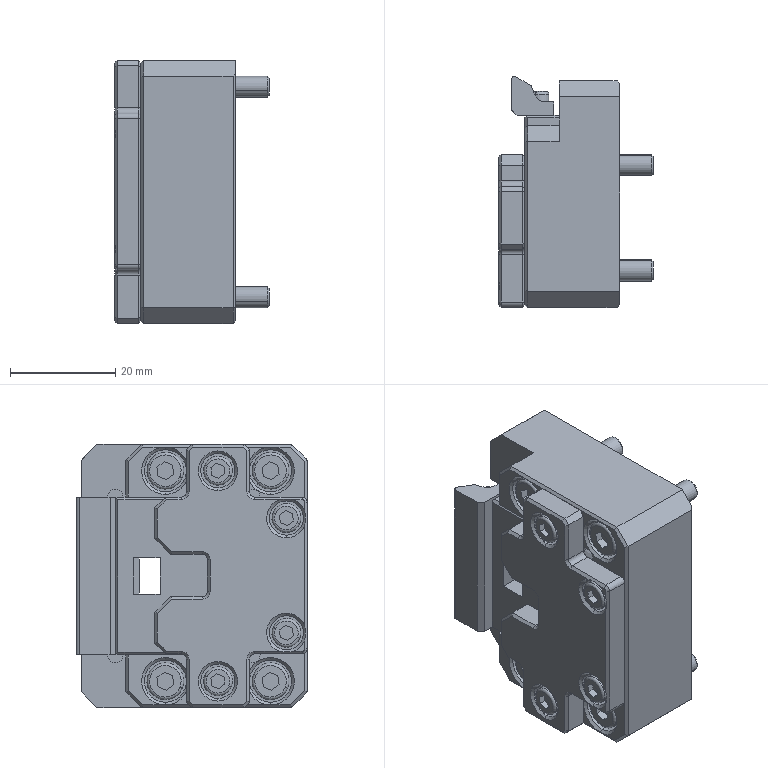Part | SolidWorks | features ReferencePattern 2, Attribute 1, CompositeCurve 1, MirrorCompFeat 1 | 18 solids | 640 faces | box 29.4 x 43.863 x 50 mm | volume 36205 mm3 | plane 279 | cylinder 169 | cone 124 | torus 60 | sphere 8 | commonest cylinder face diameters 3 x34 4 x23 2 x20 6.5 x15 2.5 x8 3.4 x8